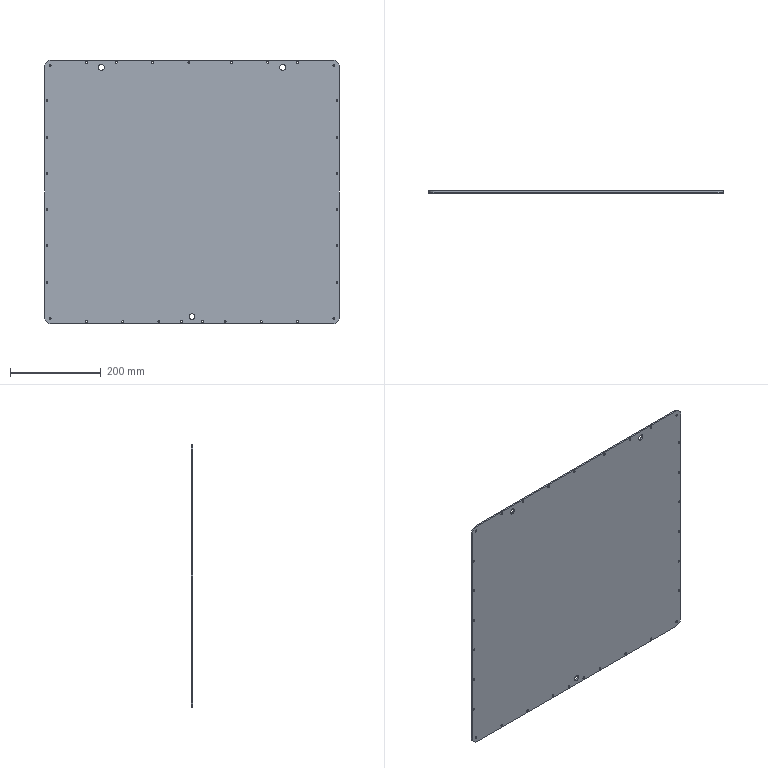Part | SolidWorks | features Extrusion 1, HoleWzd 1, ICE 1 | 1 solid | 140 faces | box 650 x 3.5 x 582 mm | volume 1318505 mm3 | cylinder 72 | cone 62 | plane 6 | commonest cylinder face diameters 4.3 x62 13 x6 30 x4